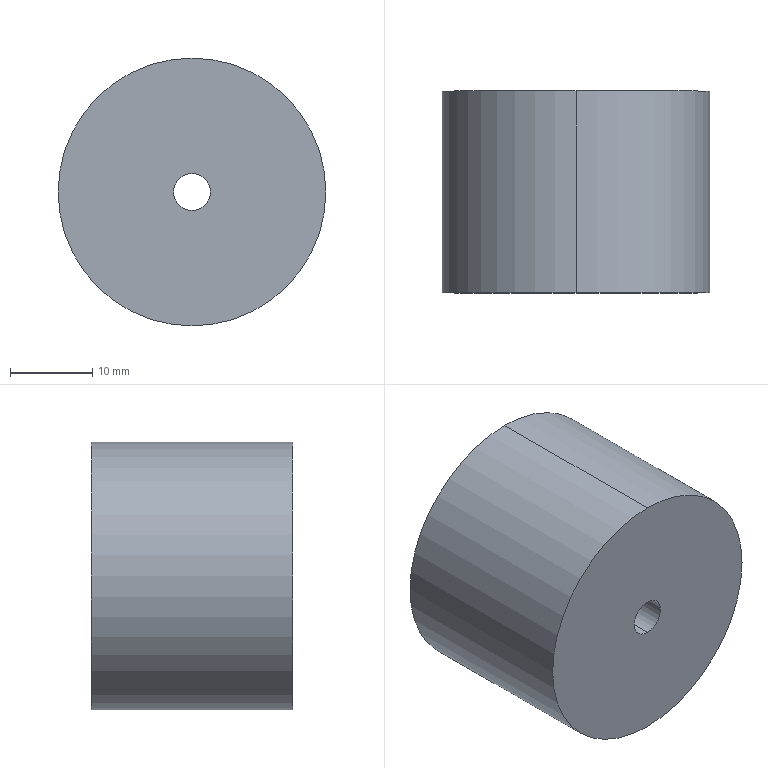Part | STEP file | PN_0041 | 1 solid | 9 faces | box 32.5 x 24.5 x 32.5 mm | volume 9394 mm3 | cylinder 6 | plane 3 | commonest cylinder face diameters 4.5 x2 27.6 x2 32.5 x2
STEP:
#1=CARTESIAN_POINT('',(0.,0.,0.));
#2=DIRECTION('',(0.,0.,1.));
#3=DIRECTION('',(1.,0.,0.));
#4=AXIS2_PLACEMENT_3D('',#1,#2,#3);
#5=CARTESIAN_POINT('',(0.,0.,2.25));
#6=VERTEX_POINT('',#5);
#7=CARTESIAN_POINT('',(0.,6.4,2.25));
#8=VERTEX_POINT('',#7);
#9=CARTESIAN_POINT('',(0.,6.4,2.25));
#10=DIRECTION('',(0.,1.,0.));
#11=VECTOR('',#10,1.);
#12=LINE('',#9,#11);
#13=CARTESIAN_POINT('',(0.,6.4,0.));
#14=DIRECTION('',(0.,1.,0.));
#15=DIRECTION('',(0.,0.,1.));
#16=AXIS2_PLACEMENT_3D('',#13,#14,#15);
#17=CYLINDRICAL_SURFACE('',#16,2.25);
#18=CARTESIAN_POINT('',(6.283,0.));
#19=DIRECTION('',(0.,1.));
#20=VECTOR('',#19,1.);
#21=LINE('',#18,#20);
#22=(GEOMETRIC_REPRESENTATION_CONTEXT(2)PARAMETRIC_REPRESENTATION_CONTEXT()REPRESENTATION_CONTEXT('',''));
#23=DEFINITIONAL_REPRESENTATION('',(#21),#22);
#24=PCURVE('',#17,#23);
#25=CARTESIAN_POINT('',(0.,6.4,0.));
#26=DIRECTION('',(0.,1.,0.));
#27=DIRECTION('',(0.,0.,1.));
#28=AXIS2_PLACEMENT_3D('',#25,#26,#27);
#29=CYLINDRICAL_SURFACE('',#28,2.25);
#30=CARTESIAN_POINT('',(0.,0.));
#31=DIRECTION('',(0.,1.));
#32=VECTOR('',#31,1.);
#33=LINE('',#30,#32);
#34=(GEOMETRIC_REPRESENTATION_CONTEXT(2)PARAMETRIC_REPRESENTATION_CONTEXT()REPRESENTATION_CONTEXT('',''));
#35=DEFINITIONAL_REPRESENTATION('',(#33),#34);
#36=PCURVE('',#29,#35);
#37=SURFACE_CURVE('',#12,(#24,#36),.PCURVE_S1.);
#38=EDGE_CURVE('',#6,#8,#37,.T.);
#39=ORIENTED_EDGE('',*,*,#38,.T.);
#40=CARTESIAN_POINT('',(0.,6.4,-2.25));
#41=VERTEX_POINT('',#40);
#42=CARTESIAN_POINT('',(0.,6.4,0.));
#43=DIRECTION('',(0.,1.,0.));
#44=DIRECTION('',(0.,0.,1.));
#45=AXIS2_PLACEMENT_3D('',#42,#43,#44);
#46=CIRCLE('',#45,2.25);
#47=CARTESIAN_POINT('',(0.,0.));
#48=DIRECTION('',(1.,0.));
#49=VECTOR('',#48,1.);
#50=LINE('',#47,#49);
#51=(GEOMETRIC_REPRESENTATION_CONTEXT(2)PARAMETRIC_REPRESENTATION_CONTEXT()REPRESENTATION_CONTEXT('',''));
#52=DEFINITIONAL_REPRESENTATION('',(#50),#51);
#53=PCURVE('',#17,#52);
#54=CARTESIAN_POINT('',(0.,6.4,0.));
#55=DIRECTION('',(0.,1.,0.));
#56=DIRECTION('',(0.,0.,1.));
#57=AXIS2_PLACEMENT_3D('',#54,#55,#56);
#58=PLANE('',#57);
#59=CARTESIAN_POINT('',(0.,0.));
#60=DIRECTION('',(1.,0.));
#61=AXIS2_PLACEMENT_2D('',#59,#60);
#62=CIRCLE('',#61,2.25);
#63=(GEOMETRIC_REPRESENTATION_CONTEXT(2)PARAMETRIC_REPRESENTATION_CONTEXT()REPRESENTATION_CONTEXT('',''));
#64=DEFINITIONAL_REPRESENTATION('',(#62),#63);
#65=PCURVE('',#58,#64);
#66=SURFACE_CURVE('',#46,(#53,#65),.PCURVE_S1.);
#67=EDGE_CURVE('',#41,#8,#66,.T.);
#68=ORIENTED_EDGE('',*,*,#67,.F.);
#69=CARTESIAN_POINT('',(0.,0.,-2.25));
#70=VERTEX_POINT('',#69);
#71=CARTESIAN_POINT('',(0.,6.4,-2.25));
#72=DIRECTION('',(0.,1.,0.));
#73=VECTOR('',#72,1.);
#74=LINE('',#71,#73);
#75=CARTESIAN_POINT('',(3.142,0.));
#76=DIRECTION('',(0.,1.));
#77=VECTOR('',#76,1.);
#78=LINE('',#75,#77);
#79=(GEOMETRIC_REPRESENTATION_CONTEXT(2)PARAMETRIC_REPRESENTATION_CONTEXT()REPRESENTATION_CONTEXT('',''));
#80=DEFINITIONAL_REPRESENTATION('',(#78),#79);
#81=PCURVE('',#17,#80);
#82=CARTESIAN_POINT('',(3.142,0.));
#83=DIRECTION('',(0.,1.));
#84=VECTOR('',#83,1.);
#85=LINE('',#82,#84);
#86=(GEOMETRIC_REPRESENTATION_CONTEXT(2)PARAMETRIC_REPRESENTATION_CONTEXT()REPRESENTATION_CONTEXT('',''));
#87=DEFINITIONAL_REPRESENTATION('',(#85),#86);
#88=PCURVE('',#29,#87);
#89=SURFACE_CURVE('',#74,(#81,#88),.PCURVE_S1.);
#90=EDGE_CURVE('',#70,#41,#89,.T.);
#91=ORIENTED_EDGE('',*,*,#90,.F.);
#92=CARTESIAN_POINT('',(0.,0.,0.));
#93=DIRECTION('',(0.,1.,0.));
#94=DIRECTION('',(0.,0.,1.));
#95=AXIS2_PLACEMENT_3D('',#92,#93,#94);
#96=CIRCLE('',#95,2.25);
#97=CARTESIAN_POINT('',(0.,-6.4));
#98=DIRECTION('',(1.,0.));
#99=VECTOR('',#98,1.);
#100=LINE('',#97,#99);
#101=(GEOMETRIC_REPRESENTATION_CONTEXT(2)PARAMETRIC_REPRESENTATION_CONTEXT()REPRESENTATION_CONTEXT('',''));
#102=DEFINITIONAL_REPRESENTATION('',(#100),#101);
#103=PCURVE('',#17,#102);
#104=CARTESIAN_POINT('',(0.,0.,0.));
#105=DIRECTION('',(0.,1.,0.));
#106=DIRECTION('',(0.,0.,1.));
#107=AXIS2_PLACEMENT_3D('',#104,#105,#106);
#108=PLANE('',#107);
#109=CARTESIAN_POINT('',(0.,0.));
#110=DIRECTION('',(1.,0.));
#111=AXIS2_PLACEMENT_2D('',#109,#110);
#112=CIRCLE('',#111,2.25);
#113=(GEOMETRIC_REPRESENTATION_CONTEXT(2)PARAMETRIC_REPRESENTATION_CONTEXT()REPRESENTATION_CONTEXT('',''));
#114=DEFINITIONAL_REPRESENTATION('',(#112),#113);
#115=PCURVE('',#108,#114);
#116=SURFACE_CURVE('',#96,(#103,#115),.PCURVE_S1.);
#117=EDGE_CURVE('',#70,#6,#116,.T.);
#118=ORIENTED_EDGE('',*,*,#117,.T.);
#119=EDGE_LOOP('',(#39,#68,#91,#118));
#120=FACE_BOUND('',#119,.F.);
#121=ADVANCED_FACE('',(#120),#17,.F.);
#122=CARTESIAN_POINT('',(0.,6.4,13.8));
#123=VERTEX_POINT('',#122);
#124=CARTESIAN_POINT('',(0.,24.5,13.8));
#125=VERTEX_POINT('',#124);
#126=CARTESIAN_POINT('',(0.,6.4,13.8));
#127=DIRECTION('',(0.,1.,0.));
#128=VECTOR('',#127,1.);
#129=LINE('',#126,#128);
#130=CARTESIAN_POINT('',(0.,6.4,0.));
#131=DIRECTION('',(0.,1.,0.));
#132=DIRECTION('',(0.,0.,1.));
#133=AXIS2_PLACEMENT_3D('',#130,#131,#132);
#134=CYLINDRICAL_SURFACE('',#133,13.8);
#135=CARTESIAN_POINT('',(6.283,0.));
#136=DIRECTION('',(0.,1.));
#137=VECTOR('',#136,1.);
#138=LINE('',#135,#137);
#139=(GEOMETRIC_REPRESENTATION_CONTEXT(2)PARAMETRIC_REPRESENTATION_CONTEXT()REPRESENTATION_CONTEXT('',''));
#140=DEFINITIONAL_REPRESENTATION('',(#138),#139);
#141=PCURVE('',#134,#140);
#142=CARTESIAN_POINT('',(0.,6.4,0.));
#143=DIRECTION('',(0.,1.,0.));
#144=DIRECTION('',(0.,0.,1.));
#145=AXIS2_PLACEMENT_3D('',#142,#143,#144);
#146=CYLINDRICAL_SURFACE('',#145,13.8);
#147=CARTESIAN_POINT('',(0.,0.));
#148=DIRECTION('',(0.,1.));
#149=VECTOR('',#148,1.);
#150=LINE('',#147,#149);
#151=(GEOMETRIC_REPRESENTATION_CONTEXT(2)PARAMETRIC_REPRESENTATION_CONTEXT()REPRESENTATION_CONTEXT('',''));
#152=DEFINITIONAL_REPRESENTATION('',(#150),#151);
#153=PCURVE('',#146,#152);
#154=SURFACE_CURVE('',#129,(#141,#153),.PCURVE_S1.);
#155=EDGE_CURVE('',#123,#125,#154,.T.);
#156=ORIENTED_EDGE('',*,*,#155,.T.);
#157=CARTESIAN_POINT('',(0.,24.5,-13.8));
#158=VERTEX_POINT('',#157);
#159=CARTESIAN_POINT('',(0.,24.5,0.));
#160=DIRECTION('',(0.,1.,0.));
#161=DIRECTION('',(0.,0.,1.));
#162=AXIS2_PLACEMENT_3D('',#159,#160,#161);
#163=CIRCLE('',#162,13.8);
#164=CARTESIAN_POINT('',(0.,18.1));
#165=DIRECTION('',(1.,0.));
#166=VECTOR('',#165,1.);
#167=LINE('',#164,#166);
#168=(GEOMETRIC_REPRESENTATION_CONTEXT(2)PARAMETRIC_REPRESENTATION_CONTEXT()REPRESENTATION_CONTEXT('',''));
#169=DEFINITIONAL_REPRESENTATION('',(#167),#168);
#170=PCURVE('',#134,#169);
#171=CARTESIAN_POINT('',(0.,24.5,0.));
#172=DIRECTION('',(0.,1.,0.));
#173=DIRECTION('',(0.,0.,1.));
#174=AXIS2_PLACEMENT_3D('',#171,#172,#173);
#175=PLANE('',#174);
#176=CARTESIAN_POINT('',(0.,0.));
#177=DIRECTION('',(1.,0.));
#178=AXIS2_PLACEMENT_2D('',#176,#177);
#179=CIRCLE('',#178,13.8);
#180=(GEOMETRIC_REPRESENTATION_CONTEXT(2)PARAMETRIC_REPRESENTATION_CONTEXT()REPRESENTATION_CONTEXT('',''));
#181=DEFINITIONAL_REPRESENTATION('',(#179),#180);
#182=PCURVE('',#175,#181);
#183=SURFACE_CURVE('',#163,(#170,#182),.PCURVE_S1.);
#184=EDGE_CURVE('',#158,#125,#183,.T.);
#185=ORIENTED_EDGE('',*,*,#184,.F.);
#186=CARTESIAN_POINT('',(0.,6.4,-13.8));
#187=VERTEX_POINT('',#186);
#188=CARTESIAN_POINT('',(0.,6.4,-13.8));
#189=DIRECTION('',(0.,1.,0.));
#190=VECTOR('',#189,1.);
#191=LINE('',#188,#190);
#192=CARTESIAN_POINT('',(3.142,0.));
#193=DIRECTION('',(0.,1.));
#194=VECTOR('',#193,1.);
#195=LINE('',#192,#194);
#196=(GEOMETRIC_REPRESENTATION_CONTEXT(2)PARAMETRIC_REPRESENTATION_CONTEXT()REPRESENTATION_CONTEXT('',''));
#197=DEFINITIONAL_REPRESENTATION('',(#195),#196);
#198=PCURVE('',#134,#197);
#199=CARTESIAN_POINT('',(3.142,0.));
#200=DIRECTION('',(0.,1.));
#201=VECTOR('',#200,1.);
#202=LINE('',#199,#201);
#203=(GEOMETRIC_REPRESENTATION_CONTEXT(2)PARAMETRIC_REPRESENTATION_CONTEXT()REPRESENTATION_CONTEXT('',''));
#204=DEFINITIONAL_REPRESENTATION('',(#202),#203);
#205=PCURVE('',#146,#204);
#206=SURFACE_CURVE('',#191,(#198,#205),.PCURVE_S1.);
#207=EDGE_CURVE('',#187,#158,#206,.T.);
#208=ORIENTED_EDGE('',*,*,#207,.F.);
#209=CARTESIAN_POINT('',(0.,6.4,0.));
#210=DIRECTION('',(0.,1.,0.));
#211=DIRECTION('',(0.,0.,1.));
#212=AXIS2_PLACEMENT_3D('',#209,#210,#211);
#213=CIRCLE('',#212,13.8);
#214=CARTESIAN_POINT('',(0.,0.));
#215=DIRECTION('',(1.,0.));
#216=VECTOR('',#215,1.);
#217=LINE('',#214,#216);
#218=(GEOMETRIC_REPRESENTATION_CONTEXT(2)PARAMETRIC_REPRESENTATION_CONTEXT()REPRESENTATION_CONTEXT('',''));
#219=DEFINITIONAL_REPRESENTATION('',(#217),#218);
#220=PCURVE('',#134,#219);
#221=CARTESIAN_POINT('',(0.,0.));
#222=DIRECTION('',(1.,0.));
#223=AXIS2_PLACEMENT_2D('',#221,#222);
#224=CIRCLE('',#223,13.8);
#225=(GEOMETRIC_REPRESENTATION_CONTEXT(2)PARAMETRIC_REPRESENTATION_CONTEXT()REPRESENTATION_CONTEXT('',''));
#226=DEFINITIONAL_REPRESENTATION('',(#224),#225);
#227=PCURVE('',#58,#226);
#228=SURFACE_CURVE('',#213,(#220,#227),.PCURVE_S1.);
#229=EDGE_CURVE('',#187,#123,#228,.T.);
#230=ORIENTED_EDGE('',*,*,#229,.T.);
#231=EDGE_LOOP('',(#156,#185,#208,#230));
#232=FACE_BOUND('',#231,.F.);
#233=ADVANCED_FACE('',(#232),#134,.F.);
#234=CARTESIAN_POINT('',(0.,24.5,16.25));
#235=VERTEX_POINT('',#234);
#236=CARTESIAN_POINT('',(0.,24.5,-16.25));
#237=VERTEX_POINT('',#236);
#238=CARTESIAN_POINT('',(0.,24.5,0.));
#239=DIRECTION('',(0.,1.,0.));
#240=DIRECTION('',(0.,0.,1.));
#241=AXIS2_PLACEMENT_3D('',#238,#239,#240);
#242=CIRCLE('',#241,16.25);
#243=CARTESIAN_POINT('',(0.,24.5,0.));
#244=DIRECTION('',(0.,-1.,0.));
#245=DIRECTION('',(0.,0.,-1.));
#246=AXIS2_PLACEMENT_3D('',#243,#244,#245);
#247=CYLINDRICAL_SURFACE('',#246,16.25);
#248=CARTESIAN_POINT('',(3.142,0.));
#249=DIRECTION('',(-1.,0.));
#250=VECTOR('',#249,1.);
#251=LINE('',#248,#250);
#252=(GEOMETRIC_REPRESENTATION_CONTEXT(2)PARAMETRIC_REPRESENTATION_CONTEXT()REPRESENTATION_CONTEXT('',''));
#253=DEFINITIONAL_REPRESENTATION('',(#251),#252);
#254=PCURVE('',#247,#253);
#255=CARTESIAN_POINT('',(0.,0.));
#256=DIRECTION('',(1.,0.));
#257=AXIS2_PLACEMENT_2D('',#255,#256);
#258=CIRCLE('',#257,16.25);
#259=(GEOMETRIC_REPRESENTATION_CONTEXT(2)PARAMETRIC_REPRESENTATION_CONTEXT()REPRESENTATION_CONTEXT('',''));
#260=DEFINITIONAL_REPRESENTATION('',(#258),#259);
#261=PCURVE('',#175,#260);
#262=SURFACE_CURVE('',#242,(#254,#261),.PCURVE_S1.);
#263=EDGE_CURVE('',#235,#237,#262,.T.);
#264=ORIENTED_EDGE('',*,*,#263,.F.);
#265=CARTESIAN_POINT('',(0.,0.,16.25));
#266=VERTEX_POINT('',#265);
#267=CARTESIAN_POINT('',(0.,24.5,16.25));
#268=DIRECTION('',(0.,-1.,0.));
#269=VECTOR('',#268,1.);
#270=LINE('',#267,#269);
#271=CARTESIAN_POINT('',(3.142,0.));
#272=DIRECTION('',(0.,1.));
#273=VECTOR('',#272,1.);
#274=LINE('',#271,#273);
#275=(GEOMETRIC_REPRESENTATION_CONTEXT(2)PARAMETRIC_REPRESENTATION_CONTEXT()REPRESENTATION_CONTEXT('',''));
#276=DEFINITIONAL_REPRESENTATION('',(#274),#275);
#277=PCURVE('',#247,#276);
#278=CARTESIAN_POINT('',(0.,24.5,0.));
#279=DIRECTION('',(0.,-1.,0.));
#280=DIRECTION('',(0.,0.,-1.));
#281=AXIS2_PLACEMENT_3D('',#278,#279,#280);
#282=CYLINDRICAL_SURFACE('',#281,16.25);
#283=CARTESIAN_POINT('',(3.142,0.));
#284=DIRECTION('',(0.,1.));
#285=VECTOR('',#284,1.);
#286=LINE('',#283,#285);
#287=(GEOMETRIC_REPRESENTATION_CONTEXT(2)PARAMETRIC_REPRESENTATION_CONTEXT()REPRESENTATION_CONTEXT('',''));
#288=DEFINITIONAL_REPRESENTATION('',(#286),#287);
#289=PCURVE('',#282,#288);
#290=SURFACE_CURVE('',#270,(#277,#289),.PCURVE_S1.);
#291=EDGE_CURVE('',#235,#266,#290,.T.);
#292=ORIENTED_EDGE('',*,*,#291,.T.);
#293=CARTESIAN_POINT('',(0.,0.,-16.25));
#294=VERTEX_POINT('',#293);
#295=CARTESIAN_POINT('',(0.,0.,0.));
#296=DIRECTION('',(0.,1.,0.));
#297=DIRECTION('',(0.,0.,1.));
#298=AXIS2_PLACEMENT_3D('',#295,#296,#297);
#299=CIRCLE('',#298,16.25);
#300=CARTESIAN_POINT('',(3.142,24.5));
#301=DIRECTION('',(-1.,0.));
#302=VECTOR('',#301,1.);
#303=LINE('',#300,#302);
#304=(GEOMETRIC_REPRESENTATION_CONTEXT(2)PARAMETRIC_REPRESENTATION_CONTEXT()REPRESENTATION_CONTEXT('',''));
#305=DEFINITIONAL_REPRESENTATION('',(#303),#304);
#306=PCURVE('',#247,#305);
#307=CARTESIAN_POINT('',(0.,0.));
#308=DIRECTION('',(1.,0.));
#309=AXIS2_PLACEMENT_2D('',#307,#308);
#310=CIRCLE('',#309,16.25);
#311=(GEOMETRIC_REPRESENTATION_CONTEXT(2)PARAMETRIC_REPRESENTATION_CONTEXT()REPRESENTATION_CONTEXT('',''));
#312=DEFINITIONAL_REPRESENTATION('',(#310),#311);
#313=PCURVE('',#108,#312);
#314=SURFACE_CURVE('',#299,(#306,#313),.PCURVE_S1.);
#315=EDGE_CURVE('',#266,#294,#314,.T.);
#316=ORIENTED_EDGE('',*,*,#315,.T.);
#317=CARTESIAN_POINT('',(0.,24.5,-16.25));
#318=DIRECTION('',(0.,-1.,0.));
#319=VECTOR('',#318,1.);
#320=LINE('',#317,#319);
#321=CARTESIAN_POINT('',(0.,0.));
#322=DIRECTION('',(0.,1.));
#323=VECTOR('',#322,1.);
#324=LINE('',#321,#323);
#325=(GEOMETRIC_REPRESENTATION_CONTEXT(2)PARAMETRIC_REPRESENTATION_CONTEXT()REPRESENTATION_CONTEXT('',''));
#326=DEFINITIONAL_REPRESENTATION('',(#324),#325);
#327=PCURVE('',#247,#326);
#328=CARTESIAN_POINT('',(6.283,0.));
#329=DIRECTION('',(0.,1.));
#330=VECTOR('',#329,1.);
#331=LINE('',#328,#330);
#332=(GEOMETRIC_REPRESENTATION_CONTEXT(2)PARAMETRIC_REPRESENTATION_CONTEXT()REPRESENTATION_CONTEXT('',''));
#333=DEFINITIONAL_REPRESENTATION('',(#331),#332);
#334=PCURVE('',#282,#333);
#335=SURFACE_CURVE('',#320,(#327,#334),.PCURVE_S1.);
#336=EDGE_CURVE('',#237,#294,#335,.T.);
#337=ORIENTED_EDGE('',*,*,#336,.F.);
#338=EDGE_LOOP('',(#264,#292,#316,#337));
#339=FACE_BOUND('',#338,.T.);
#340=ADVANCED_FACE('',(#339),#247,.T.);
#341=ORIENTED_EDGE('',*,*,#291,.F.);
#342=CARTESIAN_POINT('',(0.,24.5,0.));
#343=DIRECTION('',(0.,1.,0.));
#344=DIRECTION('',(0.,0.,1.));
#345=AXIS2_PLACEMENT_3D('',#342,#343,#344);
#346=CIRCLE('',#345,16.25);
#347=CARTESIAN_POINT('',(9.425,0.));
#348=DIRECTION('',(-1.,0.));
#349=VECTOR('',#348,1.);
#350=LINE('',#347,#349);
#351=(GEOMETRIC_REPRESENTATION_CONTEXT(2)PARAMETRIC_REPRESENTATION_CONTEXT()REPRESENTATION_CONTEXT('',''));
#352=DEFINITIONAL_REPRESENTATION('',(#350),#351);
#353=PCURVE('',#282,#352);
#354=CARTESIAN_POINT('',(0.,0.));
#355=DIRECTION('',(1.,0.));
#356=AXIS2_PLACEMENT_2D('',#354,#355);
#357=CIRCLE('',#356,16.25);
#358=(GEOMETRIC_REPRESENTATION_CONTEXT(2)PARAMETRIC_REPRESENTATION_CONTEXT()REPRESENTATION_CONTEXT('',''));
#359=DEFINITIONAL_REPRESENTATION('',(#357),#358);
#360=PCURVE('',#175,#359);
#361=SURFACE_CURVE('',#346,(#353,#360),.PCURVE_S1.);
#362=EDGE_CURVE('',#237,#235,#361,.T.);
#363=ORIENTED_EDGE('',*,*,#362,.F.);
#364=ORIENTED_EDGE('',*,*,#336,.T.);
#365=CARTESIAN_POINT('',(0.,0.,0.));
#366=DIRECTION('',(0.,1.,0.));
#367=DIRECTION('',(0.,0.,1.));
#368=AXIS2_PLACEMENT_3D('',#365,#366,#367);
#369=CIRCLE('',#368,16.25);
#370=CARTESIAN_POINT('',(9.425,24.5));
#371=DIRECTION('',(-1.,0.));
#372=VECTOR('',#371,1.);
#373=LINE('',#370,#372);
#374=(GEOMETRIC_REPRESENTATION_CONTEXT(2)PARAMETRIC_REPRESENTATION_CONTEXT()REPRESENTATION_CONTEXT('',''));
#375=DEFINITIONAL_REPRESENTATION('',(#373),#374);
#376=PCURVE('',#282,#375);
#377=CARTESIAN_POINT('',(0.,0.));
#378=DIRECTION('',(1.,0.));
#379=AXIS2_PLACEMENT_2D('',#377,#378);
#380=CIRCLE('',#379,16.25);
#381=(GEOMETRIC_REPRESENTATION_CONTEXT(2)PARAMETRIC_REPRESENTATION_CONTEXT()REPRESENTATION_CONTEXT('',''));
#382=DEFINITIONAL_REPRESENTATION('',(#380),#381);
#383=PCURVE('',#108,#382);
#384=SURFACE_CURVE('',#369,(#376,#383),.PCURVE_S1.);
#385=EDGE_CURVE('',#294,#266,#384,.T.);
#386=ORIENTED_EDGE('',*,*,#385,.T.);
#387=EDGE_LOOP('',(#341,#363,#364,#386));
#388=FACE_BOUND('',#387,.T.);
#389=ADVANCED_FACE('',(#388),#282,.T.);
#390=CARTESIAN_POINT('',(0.,24.5,0.));
#391=DIRECTION('',(0.,1.,0.));
#392=DIRECTION('',(0.,0.,1.));
#393=AXIS2_PLACEMENT_3D('',#390,#391,#392);
#394=CIRCLE('',#393,13.8);
#395=CARTESIAN_POINT('',(0.,0.));
#396=DIRECTION('',(1.,0.));
#397=AXIS2_PLACEMENT_2D('',#395,#396);
#398=CIRCLE('',#397,13.8);
#399=(GEOMETRIC_REPRESENTATION_CONTEXT(2)PARAMETRIC_REPRESENTATION_CONTEXT()REPRESENTATION_CONTEXT('',''));
#400=DEFINITIONAL_REPRESENTATION('',(#398),#399);
#401=PCURVE('',#175,#400);
#402=CARTESIAN_POINT('',(0.,18.1));
#403=DIRECTION('',(1.,0.));
#404=VECTOR('',#403,1.);
#405=LINE('',#402,#404);
#406=(GEOMETRIC_REPRESENTATION_CONTEXT(2)PARAMETRIC_REPRESENTATION_CONTEXT()REPRESENTATION_CONTEXT('',''));
#407=DEFINITIONAL_REPRESENTATION('',(#405),#406);
#408=PCURVE('',#146,#407);
#409=SURFACE_CURVE('',#394,(#401,#408),.PCURVE_S1.);
#410=EDGE_CURVE('',#125,#158,#409,.T.);
#411=ORIENTED_EDGE('',*,*,#410,.F.);
#412=ORIENTED_EDGE('',*,*,#184,.F.);
#413=EDGE_LOOP('',(#411,#412));
#414=FACE_BOUND('',#413,.T.);
#415=ORIENTED_EDGE('',*,*,#362,.T.);
#416=ORIENTED_EDGE('',*,*,#263,.T.);
#417=EDGE_LOOP('',(#415,#416));
#418=FACE_BOUND('',#417,.T.);
#419=ADVANCED_FACE('',(#414,#418),#175,.T.);
#420=CARTESIAN_POINT('',(0.,0.,0.));
#421=DIRECTION('',(0.,1.,0.));
#422=DIRECTION('',(0.,0.,1.));
#423=AXIS2_PLACEMENT_3D('',#420,#421,#422);
#424=CIRCLE('',#423,2.25);
#425=CARTESIAN_POINT('',(0.,0.));
#426=DIRECTION('',(1.,0.));
#427=AXIS2_PLACEMENT_2D('',#425,#426);
#428=CIRCLE('',#427,2.25);
#429=(GEOMETRIC_REPRESENTATION_CONTEXT(2)PARAMETRIC_REPRESENTATION_CONTEXT()REPRESENTATION_CONTEXT('',''));
#430=DEFINITIONAL_REPRESENTATION('',(#428),#429);
#431=PCURVE('',#108,#430);
#432=CARTESIAN_POINT('',(0.,-6.4));
#433=DIRECTION('',(1.,0.));
#434=VECTOR('',#433,1.);
#435=LINE('',#432,#434);
#436=(GEOMETRIC_REPRESENTATION_CONTEXT(2)PARAMETRIC_REPRESENTATION_CONTEXT()REPRESENTATION_CONTEXT('',''));
#437=DEFINITIONAL_REPRESENTATION('',(#435),#436);
#438=PCURVE('',#29,#437);
#439=SURFACE_CURVE('',#424,(#431,#438),.PCURVE_S1.);
#440=EDGE_CURVE('',#6,#70,#439,.T.);
#441=ORIENTED_EDGE('',*,*,#440,.T.);
#442=ORIENTED_EDGE('',*,*,#117,.T.);
#443=EDGE_LOOP('',(#441,#442));
#444=FACE_BOUND('',#443,.T.);
#445=ORIENTED_EDGE('',*,*,#385,.F.);
#446=ORIENTED_EDGE('',*,*,#315,.F.);
#447=EDGE_LOOP('',(#445,#446));
#448=FACE_BOUND('',#447,.T.);
#449=ADVANCED_FACE('',(#444,#448),#108,.F.);
#450=ORIENTED_EDGE('',*,*,#410,.F.);
#451=ORIENTED_EDGE('',*,*,#155,.F.);
#452=CARTESIAN_POINT('',(0.,6.4,0.));
#453=DIRECTION('',(0.,1.,0.));
#454=DIRECTION('',(0.,0.,1.));
#455=AXIS2_PLACEMENT_3D('',#452,#453,#454);
#456=CIRCLE('',#455,13.8);
#457=CARTESIAN_POINT('',(0.,0.));
#458=DIRECTION('',(1.,0.));
#459=VECTOR('',#458,1.);
#460=LINE('',#457,#459);
#461=(GEOMETRIC_REPRESENTATION_CONTEXT(2)PARAMETRIC_REPRESENTATION_CONTEXT()REPRESENTATION_CONTEXT('',''));
#462=DEFINITIONAL_REPRESENTATION('',(#460),#461);
#463=PCURVE('',#146,#462);
#464=CARTESIAN_POINT('',(0.,0.));
#465=DIRECTION('',(1.,0.));
#466=AXIS2_PLACEMENT_2D('',#464,#465);
#467=CIRCLE('',#466,13.8);
#468=(GEOMETRIC_REPRESENTATION_CONTEXT(2)PARAMETRIC_REPRESENTATION_CONTEXT()REPRESENTATION_CONTEXT('',''));
#469=DEFINITIONAL_REPRESENTATION('',(#467),#468);
#470=PCURVE('',#58,#469);
#471=SURFACE_CURVE('',#456,(#463,#470),.PCURVE_S1.);
#472=EDGE_CURVE('',#123,#187,#471,.T.);
#473=ORIENTED_EDGE('',*,*,#472,.T.);
#474=ORIENTED_EDGE('',*,*,#207,.T.);
#475=EDGE_LOOP('',(#450,#451,#473,#474));
#476=FACE_BOUND('',#475,.F.);
#477=ADVANCED_FACE('',(#476),#146,.F.);
#478=CARTESIAN_POINT('',(0.,6.4,0.));
#479=DIRECTION('',(0.,1.,0.));
#480=DIRECTION('',(0.,0.,1.));
#481=AXIS2_PLACEMENT_3D('',#478,#479,#480);
#482=CIRCLE('',#481,2.25);
#483=CARTESIAN_POINT('',(0.,0.));
#484=DIRECTION('',(1.,0.));
#485=AXIS2_PLACEMENT_2D('',#483,#484);
#486=CIRCLE('',#485,2.25);
#487=(GEOMETRIC_REPRESENTATION_CONTEXT(2)PARAMETRIC_REPRESENTATION_CONTEXT()REPRESENTATION_CONTEXT('',''));
#488=DEFINITIONAL_REPRESENTATION('',(#486),#487);
#489=PCURVE('',#58,#488);
#490=CARTESIAN_POINT('',(0.,0.));
#491=DIRECTION('',(1.,0.));
#492=VECTOR('',#491,1.);
#493=LINE('',#490,#492);
#494=(GEOMETRIC_REPRESENTATION_CONTEXT(2)PARAMETRIC_REPRESENTATION_CONTEXT()REPRESENTATION_CONTEXT('',''));
#495=DEFINITIONAL_REPRESENTATION('',(#493),#494);
#496=PCURVE('',#29,#495);
#497=SURFACE_CURVE('',#482,(#489,#496),.PCURVE_S1.);
#498=EDGE_CURVE('',#8,#41,#497,.T.);
#499=ORIENTED_EDGE('',*,*,#498,.F.);
#500=ORIENTED_EDGE('',*,*,#67,.F.);
#501=EDGE_LOOP('',(#499,#500));
#502=FACE_BOUND('',#501,.T.);
#503=ORIENTED_EDGE('',*,*,#472,.T.);
#504=ORIENTED_EDGE('',*,*,#229,.T.);
#505=EDGE_LOOP('',(#503,#504));
#506=FACE_BOUND('',#505,.T.);
#507=ADVANCED_FACE('',(#502,#506),#58,.T.);
#508=ORIENTED_EDGE('',*,*,#498,.F.);
#509=ORIENTED_EDGE('',*,*,#38,.F.);
#510=ORIENTED_EDGE('',*,*,#440,.T.);
#511=ORIENTED_EDGE('',*,*,#90,.T.);
#512=EDGE_LOOP('',(#508,#509,#510,#511));
#513=FACE_BOUND('',#512,.F.);
#514=ADVANCED_FACE('',(#513),#29,.F.);
#515=CLOSED_SHELL('',(#121,#233,#340,#389,#419,#449,#477,#507,#514));
#516=MANIFOLD_SOLID_BREP('',#515);
#517=(LENGTH_UNIT()NAMED_UNIT(*)SI_UNIT(.MILLI.,.METRE.));
#518=UNCERTAINTY_MEASURE_WITH_UNIT(LENGTH_MEASURE(0.0000001),#517,'','');
#519=(NAMED_UNIT(*)PLANE_ANGLE_UNIT()SI_UNIT($,.RADIAN.));
#520=(NAMED_UNIT(*)SI_UNIT($,.STERADIAN.)SOLID_ANGLE_UNIT());
#521=(GEOMETRIC_REPRESENTATION_CONTEXT(3)GLOBAL_UNCERTAINTY_ASSIGNED_CONTEXT((#518))GLOBAL_UNIT_ASSIGNED_CONTEXT((#517,#519,#520))REPRESENTATION_CONTEXT('',''));
#522=ADVANCED_BREP_SHAPE_REPRESENTATION('',(#4,#516),#521);